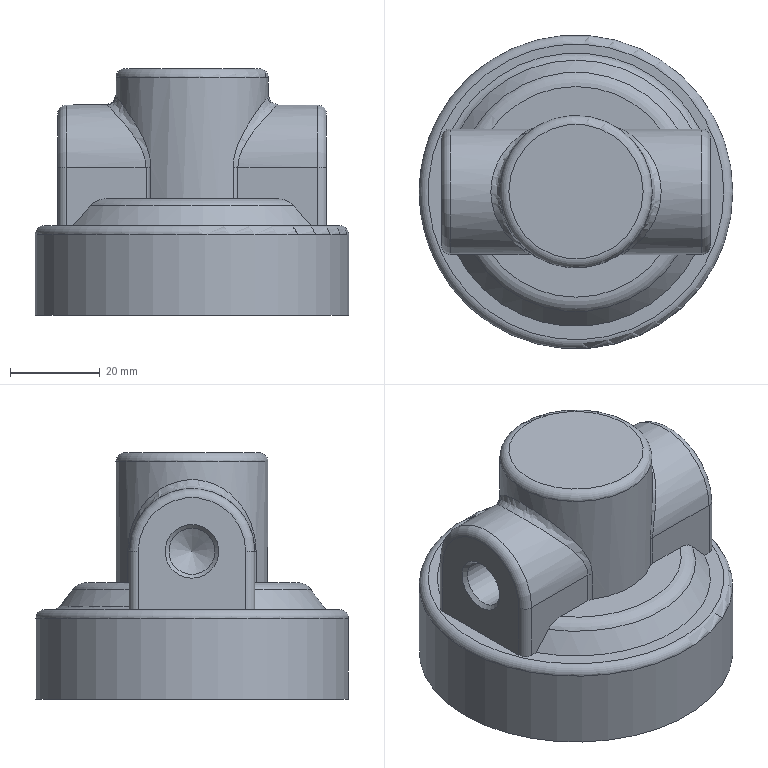Part | NX | features CYLINDER 5, HOLE PACKAGE 5, SIMPLE HOLE 5, SYMBOLIC_THREAD 4, BLEND 3, DATUM_CSYS 2, BLOCK 1, SKETCH 1, SWP104 1 | 1 solid | 51 faces | box 70 x 70 x 55 mm | volume 79994 mm3 | cylinder 19 | plane 14 | cone 9 | torus 7 | spline 2 | commonest cylinder face diameters 4 x8 10.3 x2 28 x2 3 x1 8.5 x1 34 x1
STEP:
#1=CARTESIAN_POINT('',(17.,0.,53.));
#2=VERTEX_POINT('',#1);
#3=CARTESIAN_POINT('',(0.,0.,53.));
#4=DIRECTION('',(0.,0.,1.));
#5=DIRECTION('',(1.,0.,0.));
#6=AXIS2_PLACEMENT_3D('',#3,#4,#5);
#7=CIRCLE('',#6,17.);
#8=EDGE_CURVE('',#2,#2,#7,.F.);
#9=ORIENTED_EDGE('',*,*,#8,.T.);
#10=EDGE_LOOP('',(#9));
#11=FACE_BOUND('',#10,.T.);
#12=CARTESIAN_POINT('',(9.168,-14.316,33.));
#13=VERTEX_POINT('',#12);
#14=CARTESIAN_POINT('',(9.168,14.316,33.));
#15=VERTEX_POINT('',#14);
#16=CARTESIAN_POINT('',(9.168,-14.316,33.));
#17=CARTESIAN_POINT('',(9.168,-14.316,35.135));
#18=CARTESIAN_POINT('',(10.446,-13.543,39.204));
#19=CARTESIAN_POINT('',(13.437,-10.75,44.088));
#20=CARTESIAN_POINT('',(16.145,-6.304,47.881));
#21=CARTESIAN_POINT('',(17.424,-0.02479,49.554));
#22=CARTESIAN_POINT('',(16.161,6.269,47.902));
#23=CARTESIAN_POINT('',(13.45,10.736,44.107));
#24=CARTESIAN_POINT('',(10.454,13.537,39.226));
#25=CARTESIAN_POINT('',(9.168,14.316,35.135));
#26=CARTESIAN_POINT('',(9.168,14.316,33.));
#27=B_SPLINE_CURVE_WITH_KNOTS('',3,(#16,#17,#18,#19,#20,#21,#22,#23,#24,#25,#26),.UNSPECIFIED.,.F.,.F.,(4,1,1,1,1,1,1,1,4),(0.,0.006316,0.01263,0.01895,0.02527,0.03158,0.0379,0.04422,0.05053),.UNSPECIFIED.);
#28=EDGE_CURVE('',#13,#15,#27,.T.);
#29=ORIENTED_EDGE('',*,*,#28,.T.);
#30=CARTESIAN_POINT('',(9.168,14.316,26.));
#31=VERTEX_POINT('',#30);
#32=CARTESIAN_POINT('',(9.168,14.316,0.));
#33=DIRECTION('',(0.,0.,1.));
#34=VECTOR('',#33,1000.);
#35=LINE('',#32,#34);
#36=EDGE_CURVE('',#15,#31,#35,.F.);
#37=ORIENTED_EDGE('',*,*,#36,.T.);
#38=CARTESIAN_POINT('',(-9.168,14.316,26.));
#39=VERTEX_POINT('',#38);
#40=CARTESIAN_POINT('',(0.,0.,26.));
#41=DIRECTION('',(0.,0.,-1.));
#42=DIRECTION('',(-1.,0.,0.));
#43=AXIS2_PLACEMENT_3D('',#40,#41,#42);
#44=CIRCLE('',#43,17.);
#45=EDGE_CURVE('',#31,#39,#44,.F.);
#46=ORIENTED_EDGE('',*,*,#45,.T.);
#47=CARTESIAN_POINT('',(-9.168,14.316,33.));
#48=VERTEX_POINT('',#47);
#49=CARTESIAN_POINT('',(-9.168,14.316,0.));
#50=DIRECTION('',(0.,0.,1.));
#51=VECTOR('',#50,1000.);
#52=LINE('',#49,#51);
#53=EDGE_CURVE('',#39,#48,#52,.T.);
#54=ORIENTED_EDGE('',*,*,#53,.T.);
#55=CARTESIAN_POINT('',(-9.168,-14.316,33.));
#56=VERTEX_POINT('',#55);
#57=CARTESIAN_POINT('',(-9.168,14.316,33.));
#58=CARTESIAN_POINT('',(-9.168,14.316,35.135));
#59=CARTESIAN_POINT('',(-10.446,13.543,39.204));
#60=CARTESIAN_POINT('',(-13.437,10.75,44.088));
#61=CARTESIAN_POINT('',(-16.145,6.304,47.881));
#62=CARTESIAN_POINT('',(-17.424,0.02479,49.554));
#63=CARTESIAN_POINT('',(-16.161,-6.269,47.902));
#64=CARTESIAN_POINT('',(-13.45,-10.736,44.107));
#65=CARTESIAN_POINT('',(-10.454,-13.537,39.226));
#66=CARTESIAN_POINT('',(-9.168,-14.316,35.135));
#67=CARTESIAN_POINT('',(-9.168,-14.316,33.));
#68=B_SPLINE_CURVE_WITH_KNOTS('',3,(#57,#58,#59,#60,#61,#62,#63,#64,#65,#66,#67),.UNSPECIFIED.,.F.,.F.,(4,1,1,1,1,1,1,1,4),(0.,0.006316,0.01263,0.01895,0.02527,0.03158,0.0379,0.04422,0.05053),.UNSPECIFIED.);
#69=EDGE_CURVE('',#48,#56,#68,.T.);
#70=ORIENTED_EDGE('',*,*,#69,.T.);
#71=CARTESIAN_POINT('',(-9.168,-14.316,26.));
#72=VERTEX_POINT('',#71);
#73=CARTESIAN_POINT('',(-9.168,-14.316,0.));
#74=DIRECTION('',(0.,0.,1.));
#75=VECTOR('',#74,1000.);
#76=LINE('',#73,#75);
#77=EDGE_CURVE('',#56,#72,#76,.F.);
#78=ORIENTED_EDGE('',*,*,#77,.T.);
#79=CARTESIAN_POINT('',(9.168,-14.316,26.));
#80=VERTEX_POINT('',#79);
#81=CARTESIAN_POINT('',(0.,0.,26.));
#82=DIRECTION('',(0.,0.,-1.));
#83=DIRECTION('',(-1.,0.,0.));
#84=AXIS2_PLACEMENT_3D('',#81,#82,#83);
#85=CIRCLE('',#84,17.);
#86=EDGE_CURVE('',#72,#80,#85,.F.);
#87=ORIENTED_EDGE('',*,*,#86,.T.);
#88=CARTESIAN_POINT('',(9.168,-14.316,0.));
#89=DIRECTION('',(0.,0.,1.));
#90=VECTOR('',#89,1000.);
#91=LINE('',#88,#90);
#92=EDGE_CURVE('',#80,#13,#91,.T.);
#93=ORIENTED_EDGE('',*,*,#92,.T.);
#94=EDGE_LOOP('',(#29,#37,#46,#54,#70,#78,#87,#93));
#95=FACE_BOUND('',#94,.T.);
#96=CARTESIAN_POINT('',(0.,0.,0.));
#97=DIRECTION('',(0.,0.,1.));
#98=DIRECTION('',(1.,0.,0.));
#99=AXIS2_PLACEMENT_3D('',#96,#97,#98);
#100=CYLINDRICAL_SURFACE('',#99,17.);
#101=ADVANCED_FACE('',(#11,#95),#100,.T.);
#102=CARTESIAN_POINT('',(26.533,-14.,20.));
#103=VERTEX_POINT('',#102);
#104=CARTESIAN_POINT('',(28.,-14.,20.));
#105=VERTEX_POINT('',#104);
#106=CARTESIAN_POINT('',(0.,-14.,20.));
#107=DIRECTION('',(1.,0.,0.));
#108=VECTOR('',#107,1000.);
#109=LINE('',#106,#108);
#110=EDGE_CURVE('',#103,#105,#109,.T.);
#111=ORIENTED_EDGE('',*,*,#110,.T.);
#112=CARTESIAN_POINT('',(28.,-14.,33.));
#113=VERTEX_POINT('',#112);
#114=CARTESIAN_POINT('',(28.,-14.,0.));
#115=DIRECTION('',(0.,0.,1.));
#116=VECTOR('',#115,1000.);
#117=LINE('',#114,#116);
#118=EDGE_CURVE('',#105,#113,#117,.T.);
#119=ORIENTED_EDGE('',*,*,#118,.T.);
#120=CARTESIAN_POINT('',(10.247,-14.,33.));
#121=VERTEX_POINT('',#120);
#122=CARTESIAN_POINT('',(0.,-14.,33.));
#123=DIRECTION('',(-1.,0.,0.));
#124=VECTOR('',#123,1000.);
#125=LINE('',#122,#124);
#126=EDGE_CURVE('',#113,#121,#125,.T.);
#127=ORIENTED_EDGE('',*,*,#126,.T.);
#128=CARTESIAN_POINT('',(10.247,-14.,26.));
#129=VERTEX_POINT('',#128);
#130=CARTESIAN_POINT('',(10.247,-14.,26.));
#131=DIRECTION('',(0.,0.,-1.));
#132=VECTOR('',#131,1000.);
#133=LINE('',#130,#132);
#134=EDGE_CURVE('',#121,#129,#133,.T.);
#135=ORIENTED_EDGE('',*,*,#134,.T.);
#136=CARTESIAN_POINT('',(18.875,-14.,26.));
#137=VERTEX_POINT('',#136);
#138=CARTESIAN_POINT('',(0.,-14.,26.));
#139=DIRECTION('',(1.,0.,0.));
#140=VECTOR('',#139,1000.);
#141=LINE('',#138,#140);
#142=EDGE_CURVE('',#129,#137,#141,.T.);
#143=ORIENTED_EDGE('',*,*,#142,.T.);
#144=CARTESIAN_POINT('',(22.735,-14.,24.4));
#145=VERTEX_POINT('',#144);
#146=CARTESIAN_POINT('',(18.875,-14.,26.));
#147=CARTESIAN_POINT('',(20.32,-14.,26.));
#148=CARTESIAN_POINT('',(21.777,-14.,25.488));
#149=CARTESIAN_POINT('',(22.735,-14.,24.4));
#150=B_SPLINE_CURVE_WITH_KNOTS('',3,(#146,#147,#148,#149),.UNSPECIFIED.,.F.,.F.,(4,4),(0.,0.00427),.UNSPECIFIED.);
#151=EDGE_CURVE('',#137,#145,#150,.T.);
#152=ORIENTED_EDGE('',*,*,#151,.T.);
#153=CARTESIAN_POINT('',(22.735,-14.,24.4));
#154=CARTESIAN_POINT('',(24.016,-14.,22.946));
#155=CARTESIAN_POINT('',(25.28,-14.,21.477));
#156=CARTESIAN_POINT('',(26.533,-14.,20.));
#157=B_SPLINE_CURVE_WITH_KNOTS('',3,(#153,#154,#155,#156),.UNSPECIFIED.,.F.,.F.,(4,4),(0.01619,0.022),.UNSPECIFIED.);
#158=EDGE_CURVE('',#145,#103,#157,.T.);
#159=ORIENTED_EDGE('',*,*,#158,.T.);
#160=EDGE_LOOP('',(#111,#119,#127,#135,#143,#152,#159));
#161=FACE_BOUND('',#160,.T.);
#162=CARTESIAN_POINT('',(0.,-14.,0.));
#163=DIRECTION('',(0.,-1.,0.));
#164=DIRECTION('',(0.,0.,-1.));
#165=AXIS2_PLACEMENT_3D('',#162,#163,#164);
#166=PLANE('',#165);
#167=ADVANCED_FACE('',(#161),#166,.T.);
#168=CARTESIAN_POINT('',(10.247,14.,33.));
#169=VERTEX_POINT('',#168);
#170=CARTESIAN_POINT('',(28.,14.,33.));
#171=VERTEX_POINT('',#170);
#172=CARTESIAN_POINT('',(0.,14.,33.));
#173=DIRECTION('',(1.,0.,0.));
#174=VECTOR('',#173,1000.);
#175=LINE('',#172,#174);
#176=EDGE_CURVE('',#169,#171,#175,.T.);
#177=ORIENTED_EDGE('',*,*,#176,.T.);
#178=CARTESIAN_POINT('',(28.,14.,20.));
#179=VERTEX_POINT('',#178);
#180=CARTESIAN_POINT('',(28.,14.,0.));
#181=DIRECTION('',(0.,0.,1.));
#182=VECTOR('',#181,1000.);
#183=LINE('',#180,#182);
#184=EDGE_CURVE('',#171,#179,#183,.F.);
#185=ORIENTED_EDGE('',*,*,#184,.T.);
#186=CARTESIAN_POINT('',(27.659,14.,20.));
#187=VERTEX_POINT('',#186);
#188=CARTESIAN_POINT('',(0.,14.,20.));
#189=DIRECTION('',(-1.,0.,0.));
#190=VECTOR('',#189,1000.);
#191=LINE('',#188,#190);
#192=EDGE_CURVE('',#179,#187,#191,.T.);
#193=ORIENTED_EDGE('',*,*,#192,.T.);
#194=CARTESIAN_POINT('',(25.853,14.,20.8));
#195=VERTEX_POINT('',#194);
#196=CARTESIAN_POINT('',(27.659,14.,20.));
#197=CARTESIAN_POINT('',(26.974,14.,20.));
#198=CARTESIAN_POINT('',(26.298,14.,20.278));
#199=CARTESIAN_POINT('',(25.853,14.,20.8));
#200=B_SPLINE_CURVE_WITH_KNOTS('',3,(#196,#197,#198,#199),.UNSPECIFIED.,.F.,.F.,(4,4),(0.,0.002025),.UNSPECIFIED.);
#201=EDGE_CURVE('',#187,#195,#200,.T.);
#202=ORIENTED_EDGE('',*,*,#201,.T.);
#203=CARTESIAN_POINT('',(22.735,14.,24.4));
#204=VERTEX_POINT('',#203);
#205=CARTESIAN_POINT('',(25.853,14.,20.8));
#206=CARTESIAN_POINT('',(24.823,14.,22.008));
#207=CARTESIAN_POINT('',(23.784,14.,23.209));
#208=CARTESIAN_POINT('',(22.735,14.,24.4));
#209=B_SPLINE_CURVE_WITH_KNOTS('',3,(#205,#206,#207,#208),.UNSPECIFIED.,.F.,.F.,(4,4),(0.03,0.03477),.UNSPECIFIED.);
#210=EDGE_CURVE('',#195,#204,#209,.T.);
#211=ORIENTED_EDGE('',*,*,#210,.T.);
#212=CARTESIAN_POINT('',(18.875,14.,26.));
#213=VERTEX_POINT('',#212);
#214=CARTESIAN_POINT('',(22.735,14.,24.4));
#215=CARTESIAN_POINT('',(21.778,14.,25.487));
#216=CARTESIAN_POINT('',(20.318,14.,26.));
#217=CARTESIAN_POINT('',(18.875,14.,26.));
#218=B_SPLINE_CURVE_WITH_KNOTS('',3,(#214,#215,#216,#217),.UNSPECIFIED.,.F.,.F.,(4,4),(0.,0.004276),.UNSPECIFIED.);
#219=EDGE_CURVE('',#204,#213,#218,.T.);
#220=ORIENTED_EDGE('',*,*,#219,.T.);
#221=CARTESIAN_POINT('',(10.247,14.,26.));
#222=VERTEX_POINT('',#221);
#223=CARTESIAN_POINT('',(0.,14.,26.));
#224=DIRECTION('',(-1.,0.,0.));
#225=VECTOR('',#224,1000.);
#226=LINE('',#223,#225);
#227=EDGE_CURVE('',#213,#222,#226,.T.);
#228=ORIENTED_EDGE('',*,*,#227,.T.);
#229=CARTESIAN_POINT('',(10.247,14.,33.));
#230=DIRECTION('',(0.,0.,-1.));
#231=VECTOR('',#230,1000.);
#232=LINE('',#229,#231);
#233=EDGE_CURVE('',#222,#169,#232,.F.);
#234=ORIENTED_EDGE('',*,*,#233,.T.);
#235=EDGE_LOOP('',(#177,#185,#193,#202,#211,#220,#228,#234));
#236=FACE_BOUND('',#235,.T.);
#237=CARTESIAN_POINT('',(0.,14.,0.));
#238=DIRECTION('',(0.,1.,0.));
#239=DIRECTION('',(0.,0.,1.));
#240=AXIS2_PLACEMENT_3D('',#237,#238,#239);
#241=PLANE('',#240);
#242=ADVANCED_FACE('',(#236),#241,.T.);
#243=CARTESIAN_POINT('',(-27.659,14.,20.));
#244=VERTEX_POINT('',#243);
#245=CARTESIAN_POINT('',(-28.,14.,20.));
#246=VERTEX_POINT('',#245);
#247=CARTESIAN_POINT('',(0.,14.,20.));
#248=DIRECTION('',(-1.,0.,0.));
#249=VECTOR('',#248,1000.);
#250=LINE('',#247,#249);
#251=EDGE_CURVE('',#244,#246,#250,.T.);
#252=ORIENTED_EDGE('',*,*,#251,.T.);
#253=CARTESIAN_POINT('',(-28.,14.,33.));
#254=VERTEX_POINT('',#253);
#255=CARTESIAN_POINT('',(-28.,14.,0.));
#256=DIRECTION('',(0.,0.,1.));
#257=VECTOR('',#256,1000.);
#258=LINE('',#255,#257);
#259=EDGE_CURVE('',#246,#254,#258,.T.);
#260=ORIENTED_EDGE('',*,*,#259,.T.);
#261=CARTESIAN_POINT('',(-10.247,14.,33.));
#262=VERTEX_POINT('',#261);
#263=CARTESIAN_POINT('',(0.,14.,33.));
#264=DIRECTION('',(1.,0.,0.));
#265=VECTOR('',#264,1000.);
#266=LINE('',#263,#265);
#267=EDGE_CURVE('',#254,#262,#266,.T.);
#268=ORIENTED_EDGE('',*,*,#267,.T.);
#269=CARTESIAN_POINT('',(-10.247,14.,26.));
#270=VERTEX_POINT('',#269);
#271=CARTESIAN_POINT('',(-10.247,14.,26.));
#272=DIRECTION('',(0.,0.,-1.));
#273=VECTOR('',#272,1000.);
#274=LINE('',#271,#273);
#275=EDGE_CURVE('',#262,#270,#274,.T.);
#276=ORIENTED_EDGE('',*,*,#275,.T.);
#277=CARTESIAN_POINT('',(-18.875,14.,26.));
#278=VERTEX_POINT('',#277);
#279=CARTESIAN_POINT('',(0.,14.,26.));
#280=DIRECTION('',(-1.,0.,0.));
#281=VECTOR('',#280,1000.);
#282=LINE('',#279,#281);
#283=EDGE_CURVE('',#270,#278,#282,.T.);
#284=ORIENTED_EDGE('',*,*,#283,.T.);
#285=CARTESIAN_POINT('',(-22.735,14.,24.4));
#286=VERTEX_POINT('',#285);
#287=CARTESIAN_POINT('',(-18.875,14.,26.));
#288=CARTESIAN_POINT('',(-20.32,14.,26.));
#289=CARTESIAN_POINT('',(-21.777,14.,25.488));
#290=CARTESIAN_POINT('',(-22.735,14.,24.4));
#291=B_SPLINE_CURVE_WITH_KNOTS('',3,(#287,#288,#289,#290),.UNSPECIFIED.,.F.,.F.,(4,4),(0.,0.00427),.UNSPECIFIED.);
#292=EDGE_CURVE('',#278,#286,#291,.T.);
#293=ORIENTED_EDGE('',*,*,#292,.T.);
#294=CARTESIAN_POINT('',(-25.853,14.,20.8));
#295=VERTEX_POINT('',#294);
#296=CARTESIAN_POINT('',(-22.735,14.,24.4));
#297=CARTESIAN_POINT('',(-23.784,14.,23.209));
#298=CARTESIAN_POINT('',(-24.822,14.,22.008));
#299=CARTESIAN_POINT('',(-25.853,14.,20.8));
#300=B_SPLINE_CURVE_WITH_KNOTS('',3,(#296,#297,#298,#299),.UNSPECIFIED.,.F.,.F.,(4,4),(0.01405,0.01881),.UNSPECIFIED.);
#301=EDGE_CURVE('',#286,#295,#300,.T.);
#302=ORIENTED_EDGE('',*,*,#301,.T.);
#303=CARTESIAN_POINT('',(-25.853,14.,20.8));
#304=CARTESIAN_POINT('',(-26.297,14.,20.279));
#305=CARTESIAN_POINT('',(-26.975,14.,20.));
#306=CARTESIAN_POINT('',(-27.659,14.,20.));
#307=B_SPLINE_CURVE_WITH_KNOTS('',3,(#303,#304,#305,#306),.UNSPECIFIED.,.F.,.F.,(4,4),(0.,0.002024),.UNSPECIFIED.);
#308=EDGE_CURVE('',#295,#244,#307,.T.);
#309=ORIENTED_EDGE('',*,*,#308,.T.);
#310=EDGE_LOOP('',(#252,#260,#268,#276,#284,#293,#302,#309));
#311=FACE_BOUND('',#310,.T.);
#312=CARTESIAN_POINT('',(0.,14.,0.));
#313=DIRECTION('',(0.,1.,0.));
#314=DIRECTION('',(0.,0.,1.));
#315=AXIS2_PLACEMENT_3D('',#312,#313,#314);
#316=PLANE('',#315);
#317=ADVANCED_FACE('',(#311),#316,.T.);
#318=CARTESIAN_POINT('',(-10.247,-14.,33.));
#319=VERTEX_POINT('',#318);
#320=CARTESIAN_POINT('',(-28.,-14.,33.));
#321=VERTEX_POINT('',#320);
#322=CARTESIAN_POINT('',(0.,-14.,33.));
#323=DIRECTION('',(-1.,0.,0.));
#324=VECTOR('',#323,1000.);
#325=LINE('',#322,#324);
#326=EDGE_CURVE('',#319,#321,#325,.T.);
#327=ORIENTED_EDGE('',*,*,#326,.T.);
#328=CARTESIAN_POINT('',(-28.,-14.,20.));
#329=VERTEX_POINT('',#328);
#330=CARTESIAN_POINT('',(-28.,-14.,0.));
#331=DIRECTION('',(0.,0.,1.));
#332=VECTOR('',#331,1000.);
#333=LINE('',#330,#332);
#334=EDGE_CURVE('',#321,#329,#333,.F.);
#335=ORIENTED_EDGE('',*,*,#334,.T.);
#336=CARTESIAN_POINT('',(-26.533,-14.,20.));
#337=VERTEX_POINT('',#336);
#338=CARTESIAN_POINT('',(0.,-14.,20.));
#339=DIRECTION('',(1.,0.,0.));
#340=VECTOR('',#339,1000.);
#341=LINE('',#338,#340);
#342=EDGE_CURVE('',#329,#337,#341,.T.);
#343=ORIENTED_EDGE('',*,*,#342,.T.);
#344=CARTESIAN_POINT('',(-22.735,-14.,24.4));
#345=VERTEX_POINT('',#344);
#346=CARTESIAN_POINT('',(-26.533,-14.,20.));
#347=CARTESIAN_POINT('',(-25.28,-14.,21.478));
#348=CARTESIAN_POINT('',(-24.015,-14.,22.947));
#349=CARTESIAN_POINT('',(-22.735,-14.,24.4));
#350=B_SPLINE_CURVE_WITH_KNOTS('',3,(#346,#347,#348,#349),.UNSPECIFIED.,.F.,.F.,(4,4),(0.0346,0.04041),.UNSPECIFIED.);
#351=EDGE_CURVE('',#337,#345,#350,.T.);
#352=ORIENTED_EDGE('',*,*,#351,.T.);
#353=CARTESIAN_POINT('',(-18.875,-14.,26.));
#354=VERTEX_POINT('',#353);
#355=CARTESIAN_POINT('',(-22.735,-14.,24.4));
#356=CARTESIAN_POINT('',(-21.778,-14.,25.487));
#357=CARTESIAN_POINT('',(-20.318,-14.,26.));
#358=CARTESIAN_POINT('',(-18.875,-14.,26.));
#359=B_SPLINE_CURVE_WITH_KNOTS('',3,(#355,#356,#357,#358),.UNSPECIFIED.,.F.,.F.,(4,4),(0.,0.004276),.UNSPECIFIED.);
#360=EDGE_CURVE('',#345,#354,#359,.T.);
#361=ORIENTED_EDGE('',*,*,#360,.T.);
#362=CARTESIAN_POINT('',(-10.247,-14.,26.));
#363=VERTEX_POINT('',#362);
#364=CARTESIAN_POINT('',(0.,-14.,26.));
#365=DIRECTION('',(1.,0.,0.));
#366=VECTOR('',#365,1000.);
#367=LINE('',#364,#366);
#368=EDGE_CURVE('',#354,#363,#367,.T.);
#369=ORIENTED_EDGE('',*,*,#368,.T.);
#370=CARTESIAN_POINT('',(-10.247,-14.,33.));
#371=DIRECTION('',(0.,0.,-1.));
#372=VECTOR('',#371,1000.);
#373=LINE('',#370,#372);
#374=EDGE_CURVE('',#363,#319,#373,.F.);
#375=ORIENTED_EDGE('',*,*,#374,.T.);
#376=EDGE_LOOP('',(#327,#335,#343,#352,#361,#369,#375));
#377=FACE_BOUND('',#376,.T.);
#378=CARTESIAN_POINT('',(0.,-14.,0.));
#379=DIRECTION('',(0.,-1.,0.));
#380=DIRECTION('',(0.,0.,-1.));
#381=AXIS2_PLACEMENT_3D('',#378,#379,#380);
#382=PLANE('',#381);
#383=ADVANCED_FACE('',(#377),#382,.T.);
#384=CARTESIAN_POINT('',(33.,0.,20.));
#385=VERTEX_POINT('',#384);
#386=CARTESIAN_POINT('',(0.,0.,20.));
#387=DIRECTION('',(0.,0.,1.));
#388=DIRECTION('',(1.,0.,0.));
#389=AXIS2_PLACEMENT_3D('',#386,#387,#388);
#390=CIRCLE('',#389,33.);
#391=EDGE_CURVE('',#385,#385,#390,.T.);
#392=ORIENTED_EDGE('',*,*,#391,.T.);
#393=EDGE_LOOP('',(#392));
#394=FACE_BOUND('',#393,.T.);
#395=CARTESIAN_POINT('',(-30.,12.,20.));
#396=VERTEX_POINT('',#395);
#397=CARTESIAN_POINT('',(-30.,0.,20.));
#398=VERTEX_POINT('',#397);
#399=CARTESIAN_POINT('',(-30.,0.,20.));
#400=DIRECTION('',(0.,-1.,0.));
#401=VECTOR('',#400,1000.);
#402=LINE('',#399,#401);
#403=EDGE_CURVE('',#396,#398,#402,.T.);
#404=ORIENTED_EDGE('',*,*,#403,.F.);
#405=CARTESIAN_POINT('',(-28.,12.,20.));
#406=DIRECTION('',(0.,0.,1.));
#407=DIRECTION('',(1.,0.,0.));
#408=AXIS2_PLACEMENT_3D('',#405,#406,#407);
#409=CIRCLE('',#408,2.);
#410=EDGE_CURVE('',#396,#246,#409,.F.);
#411=ORIENTED_EDGE('',*,*,#410,.T.);
#412=ORIENTED_EDGE('',*,*,#251,.F.);
#413=CARTESIAN_POINT('',(0.,0.,20.));
#414=DIRECTION('',(0.,0.,1.));
#415=DIRECTION('',(1.,0.,0.));
#416=AXIS2_PLACEMENT_3D('',#413,#414,#415);
#417=CIRCLE('',#416,31.);
#418=EDGE_CURVE('',#244,#187,#417,.F.);
#419=ORIENTED_EDGE('',*,*,#418,.T.);
#420=ORIENTED_EDGE('',*,*,#192,.F.);
#421=CARTESIAN_POINT('',(30.,12.,20.));
#422=VERTEX_POINT('',#421);
#423=CARTESIAN_POINT('',(28.,12.,20.));
#424=DIRECTION('',(0.,0.,1.));
#425=DIRECTION('',(1.,0.,0.));
#426=AXIS2_PLACEMENT_3D('',#423,#424,#425);
#427=CIRCLE('',#426,2.);
#428=EDGE_CURVE('',#179,#422,#427,.F.);
#429=ORIENTED_EDGE('',*,*,#428,.T.);
#430=CARTESIAN_POINT('',(30.,0.,20.));
#431=VERTEX_POINT('',#430);
#432=CARTESIAN_POINT('',(30.,0.,20.));
#433=DIRECTION('',(0.,1.,0.));
#434=VECTOR('',#433,1000.);
#435=LINE('',#432,#434);
#436=EDGE_CURVE('',#431,#422,#435,.T.);
#437=ORIENTED_EDGE('',*,*,#436,.F.);
#438=CARTESIAN_POINT('',(30.,-12.,20.));
#439=VERTEX_POINT('',#438);
#440=CARTESIAN_POINT('',(30.,0.,20.));
#441=DIRECTION('',(0.,1.,0.));
#442=VECTOR('',#441,1000.);
#443=LINE('',#440,#442);
#444=EDGE_CURVE('',#439,#431,#443,.T.);
#445=ORIENTED_EDGE('',*,*,#444,.F.);
#446=CARTESIAN_POINT('',(28.,-12.,20.));
#447=DIRECTION('',(0.,0.,1.));
#448=DIRECTION('',(1.,0.,0.));
#449=AXIS2_PLACEMENT_3D('',#446,#447,#448);
#450=CIRCLE('',#449,2.);
#451=EDGE_CURVE('',#439,#105,#450,.F.);
#452=ORIENTED_EDGE('',*,*,#451,.T.);
#453=ORIENTED_EDGE('',*,*,#110,.F.);
#454=CARTESIAN_POINT('',(0.,0.,20.));
#455=DIRECTION('',(0.,0.,1.));
#456=DIRECTION('',(1.,0.,0.));
#457=AXIS2_PLACEMENT_3D('',#454,#455,#456);
#458=CIRCLE('',#457,30.);
#459=EDGE_CURVE('',#337,#103,#458,.T.);
#460=ORIENTED_EDGE('',*,*,#459,.F.);
#461=ORIENTED_EDGE('',*,*,#342,.F.);
#462=CARTESIAN_POINT('',(-30.,-12.,20.));
#463=VERTEX_POINT('',#462);
#464=CARTESIAN_POINT('',(-28.,-12.,20.));
#465=DIRECTION('',(0.,0.,1.));
#466=DIRECTION('',(1.,0.,0.));
#467=AXIS2_PLACEMENT_3D('',#464,#465,#466);
#468=CIRCLE('',#467,2.);
#469=EDGE_CURVE('',#329,#463,#468,.F.);
#470=ORIENTED_EDGE('',*,*,#469,.T.);
#471=CARTESIAN_POINT('',(-30.,0.,20.));
#472=DIRECTION('',(0.,-1.,0.));
#473=VECTOR('',#472,1000.);
#474=LINE('',#471,#473);
#475=EDGE_CURVE('',#398,#463,#474,.T.);
#476=ORIENTED_EDGE('',*,*,#475,.F.);
#477=EDGE_LOOP('',(#404,#411,#412,#419,#420,#429,#437,#445,#452,#453,#460,#461,#470,#476));
#478=FACE_BOUND('',#477,.T.);
#479=CARTESIAN_POINT('',(0.,0.,20.));
#480=DIRECTION('',(0.,0.,1.));
#481=DIRECTION('',(1.,0.,0.));
#482=AXIS2_PLACEMENT_3D('',#479,#480,#481);
#483=PLANE('',#482);
#484=ADVANCED_FACE('',(#394,#478),#483,.T.);
#485=CARTESIAN_POINT('',(-30.,0.,0.));
#486=VERTEX_POINT('',#485);
#487=CARTESIAN_POINT('',(0.,0.,0.));
#488=DIRECTION('',(0.,0.,-1.));
#489=DIRECTION('',(-1.,0.,0.));
#490=AXIS2_PLACEMENT_3D('',#487,#488,#489);
#491=CIRCLE('',#490,30.);
#492=EDGE_CURVE('',#486,#486,#491,.F.);
#493=ORIENTED_EDGE('',*,*,#492,.T.);
#494=EDGE_LOOP('',(#493));
#495=FACE_BOUND('',#494,.T.);
#496=CARTESIAN_POINT('',(35.,0.,0.));
#497=VERTEX_POINT('',#496);
#498=CARTESIAN_POINT('',(0.,0.,0.));
#499=DIRECTION('',(0.,0.,1.));
#500=DIRECTION('',(1.,0.,0.));
#501=AXIS2_PLACEMENT_3D('',#498,#499,#500);
#502=CIRCLE('',#501,35.);
#503=EDGE_CURVE('',#497,#497,#502,.T.);
#504=ORIENTED_EDGE('',*,*,#503,.F.);
#505=EDGE_LOOP('',(#504));
#506=FACE_BOUND('',#505,.T.);
#507=CARTESIAN_POINT('',(0.,0.,0.));
#508=DIRECTION('',(0.,0.,-1.));
#509=DIRECTION('',(-1.,0.,0.));
#510=AXIS2_PLACEMENT_3D('',#507,#508,#509);
#511=PLANE('',#510);
#512=ADVANCED_FACE('',(#495,#506),#511,.T.);
#513=CARTESIAN_POINT('',(35.,0.,18.));
#514=VERTEX_POINT('',#513);
#515=CARTESIAN_POINT('',(0.,0.,18.));
#516=DIRECTION('',(0.,0.,1.));
#517=DIRECTION('',(1.,0.,0.));
#518=AXIS2_PLACEMENT_3D('',#515,#516,#517);
#519=CIRCLE('',#518,35.);
#520=EDGE_CURVE('',#514,#514,#519,.F.);
#521=ORIENTED_EDGE('',*,*,#520,.T.);
#522=EDGE_LOOP('',(#521));
#523=FACE_BOUND('',#522,.T.);
#524=ORIENTED_EDGE('',*,*,#503,.T.);
#525=EDGE_LOOP('',(#524));
#526=FACE_BOUND('',#525,.T.);
#527=CARTESIAN_POINT('',(0.,0.,0.));
#528=DIRECTION('',(0.,0.,1.));
#529=DIRECTION('',(1.,0.,0.));
#530=AXIS2_PLACEMENT_3D('',#527,#528,#529);
#531=CYLINDRICAL_SURFACE('',#530,35.);
#532=ADVANCED_FACE('',(#523,#526),#531,.T.);
#533=CARTESIAN_POINT('',(15.,0.,55.));
#534=VERTEX_POINT('',#533);
#535=CARTESIAN_POINT('',(0.,0.,55.));
#536=DIRECTION('',(0.,0.,1.));
#537=DIRECTION('',(1.,0.,0.));
#538=AXIS2_PLACEMENT_3D('',#535,#536,#537);
#539=CIRCLE('',#538,15.);
#540=EDGE_CURVE('',#534,#534,#539,.T.);
#541=ORIENTED_EDGE('',*,*,#540,.T.);
#542=EDGE_LOOP('',(#541));
#543=FACE_BOUND('',#542,.T.);
#544=CARTESIAN_POINT('',(0.,0.,55.));
#545=DIRECTION('',(0.,0.,1.));
#546=DIRECTION('',(1.,0.,0.));
#547=AXIS2_PLACEMENT_3D('',#544,#545,#546);
#548=PLANE('',#547);
#549=ADVANCED_FACE('',(#543),#548,.T.);
#550=CARTESIAN_POINT('',(30.,0.,27.));
#551=VERTEX_POINT('',#550);
#552=CARTESIAN_POINT('',(30.,0.,33.));
#553=DIRECTION('',(1.,0.,0.));
#554=DIRECTION('',(0.,0.,-1.));
#555=AXIS2_PLACEMENT_3D('',#552,#553,#554);
#556=CIRCLE('',#555,6.);
#557=EDGE_CURVE('',#551,#551,#556,.F.);
#558=ORIENTED_EDGE('',*,*,#557,.T.);
#559=EDGE_LOOP('',(#558));
#560=FACE_BOUND('',#559,.T.);
#561=CARTESIAN_POINT('',(30.,12.,33.));
#562=VERTEX_POINT('',#561);
#563=CARTESIAN_POINT('',(30.,-12.,33.));
#564=VERTEX_POINT('',#563);
#565=CARTESIAN_POINT('',(30.,0.,33.));
#566=DIRECTION('',(1.,0.,0.));
#567=DIRECTION('',(0.,0.,-1.));
#568=AXIS2_PLACEMENT_3D('',#565,#566,#567);
#569=CIRCLE('',#568,12.);
#570=EDGE_CURVE('',#562,#564,#569,.T.);
#571=ORIENTED_EDGE('',*,*,#570,.T.);
#572=CARTESIAN_POINT('',(30.,-12.,0.));
#573=DIRECTION('',(0.,0.,1.));
#574=VECTOR('',#573,1000.);
#575=LINE('',#572,#574);
#576=EDGE_CURVE('',#564,#439,#575,.F.);
#577=ORIENTED_EDGE('',*,*,#576,.T.);
#578=ORIENTED_EDGE('',*,*,#444,.T.);
#579=ORIENTED_EDGE('',*,*,#436,.T.);
#580=CARTESIAN_POINT('',(30.,12.,0.));
#581=DIRECTION('',(0.,0.,1.));
#582=VECTOR('',#581,1000.);
#583=LINE('',#580,#582);
#584=EDGE_CURVE('',#422,#562,#583,.T.);
#585=ORIENTED_EDGE('',*,*,#584,.T.);
#586=EDGE_LOOP('',(#571,#577,#578,#579,#585));
#587=FACE_BOUND('',#586,.T.);
#588=CARTESIAN_POINT('',(30.,0.,0.));
#589=DIRECTION('',(1.,0.,0.));
#590=DIRECTION('',(0.,0.,-1.));
#591=AXIS2_PLACEMENT_3D('',#588,#589,#590);
#592=PLANE('',#591);
#593=ADVANCED_FACE('',(#560,#587),#592,.T.);
#594=CARTESIAN_POINT('',(-30.,0.,39.));
#595=VERTEX_POINT('',#594);
#596=CARTESIAN_POINT('',(-30.,0.,33.));
#597=DIRECTION('',(-1.,0.,0.));
#598=DIRECTION('',(0.,0.,1.));
#599=AXIS2_PLACEMENT_3D('',#596,#597,#598);
#600=CIRCLE('',#599,6.);
#601=EDGE_CURVE('',#595,#595,#600,.F.);
#602=ORIENTED_EDGE('',*,*,#601,.T.);
#603=EDGE_LOOP('',(#602));
#604=FACE_BOUND('',#603,.T.);
#605=CARTESIAN_POINT('',(-30.,-12.,33.));
#606=VERTEX_POINT('',#605);
#607=CARTESIAN_POINT('',(-30.,12.,33.));
#608=VERTEX_POINT('',#607);
#609=CARTESIAN_POINT('',(-30.,0.,33.));
#610=DIRECTION('',(-1.,0.,0.));
#611=DIRECTION('',(0.,0.,1.));
#612=AXIS2_PLACEMENT_3D('',#609,#610,#611);
#613=CIRCLE('',#612,12.);
#614=EDGE_CURVE('',#606,#608,#613,.T.);
#615=ORIENTED_EDGE('',*,*,#614,.T.);
#616=CARTESIAN_POINT('',(-30.,12.,0.));
#617=DIRECTION('',(0.,0.,1.));
#618=VECTOR('',#617,1000.);
#619=LINE('',#616,#618);
#620=EDGE_CURVE('',#608,#396,#619,.F.);
#621=ORIENTED_EDGE('',*,*,#620,.T.);
#622=ORIENTED_EDGE('',*,*,#403,.T.);
#623=ORIENTED_EDGE('',*,*,#475,.T.);
#624=CARTESIAN_POINT('',(-30.,-12.,0.));
#625=DIRECTION('',(0.,0.,1.));
#626=VECTOR('',#625,1000.);
#627=LINE('',#624,#626);
#628=EDGE_CURVE('',#463,#606,#627,.T.);
#629=ORIENTED_EDGE('',*,*,#628,.T.);
#630=EDGE_LOOP('',(#615,#621,#622,#623,#629));
#631=FACE_BOUND('',#630,.T.);
#632=CARTESIAN_POINT('',(-30.,0.,0.));
#633=DIRECTION('',(-1.,0.,0.));
#634=DIRECTION('',(0.,0.,1.));
#635=AXIS2_PLACEMENT_3D('',#632,#633,#634);
#636=PLANE('',#635);
#637=ADVANCED_FACE('',(#604,#631),#636,.T.);
#638=ORIENTED_EDGE('',*,*,#267,.F.);
#639=CARTESIAN_POINT('',(-28.,0.,33.));
#640=DIRECTION('',(-1.,0.,0.));
#641=DIRECTION('',(0.,0.,1.));
#642=AXIS2_PLACEMENT_3D('',#639,#640,#641);
#643=CIRCLE('',#642,14.);
#644=EDGE_CURVE('',#254,#321,#643,.F.);
#645=ORIENTED_EDGE('',*,*,#644,.T.);
#646=ORIENTED_EDGE('',*,*,#326,.F.);
#647=CARTESIAN_POINT('',(-10.247,-14.,33.));
#648=CARTESIAN_POINT('',(-10.247,-14.,35.031));
#649=CARTESIAN_POINT('',(-11.896,-13.111,38.768));
#650=CARTESIAN_POINT('',(-15.216,-10.291,42.923));
#651=CARTESIAN_POINT('',(-18.125,-5.942,46.105));
#652=CARTESIAN_POINT('',(-19.442,0.02427,47.452));
#653=CARTESIAN_POINT('',(-18.108,5.978,46.086));
#654=CARTESIAN_POINT('',(-15.201,10.306,42.907));
#655=CARTESIAN_POINT('',(-11.884,13.118,38.745));
#656=CARTESIAN_POINT('',(-10.247,14.,35.032));
#657=CARTESIAN_POINT('',(-10.247,14.,33.));
#658=B_SPLINE_CURVE_WITH_KNOTS('',3,(#647,#648,#649,#650,#651,#652,#653,#654,#655,#656,#657),.UNSPECIFIED.,.F.,.F.,(4,1,1,1,1,1,1,1,4),(0.,0.006084,0.01217,0.01825,0.02434,0.03042,0.03651,0.04259,0.04868),.UNSPECIFIED.);
#659=EDGE_CURVE('',#319,#262,#658,.T.);
#660=ORIENTED_EDGE('',*,*,#659,.T.);
#661=EDGE_LOOP('',(#638,#645,#646,#660));
#662=FACE_BOUND('',#661,.T.);
#663=CARTESIAN_POINT('',(-30.,0.,33.));
#664=DIRECTION('',(1.,0.,0.));
#665=DIRECTION('',(0.,0.,-1.));
#666=AXIS2_PLACEMENT_3D('',#663,#664,#665);
#667=CYLINDRICAL_SURFACE('',#666,14.);
#668=ADVANCED_FACE('',(#662),#667,.T.);
#669=ORIENTED_EDGE('',*,*,#126,.F.);
#670=CARTESIAN_POINT('',(28.,0.,33.));
#671=DIRECTION('',(1.,0.,0.));
#672=DIRECTION('',(0.,0.,-1.));
#673=AXIS2_PLACEMENT_3D('',#670,#671,#672);
#674=CIRCLE('',#673,14.);
#675=EDGE_CURVE('',#113,#171,#674,.F.);
#676=ORIENTED_EDGE('',*,*,#675,.T.);
#677=ORIENTED_EDGE('',*,*,#176,.F.);
#678=CARTESIAN_POINT('',(10.247,14.,33.));
#679=CARTESIAN_POINT('',(10.247,14.,35.031));
#680=CARTESIAN_POINT('',(11.896,13.111,38.768));
#681=CARTESIAN_POINT('',(15.216,10.291,42.923));
#682=CARTESIAN_POINT('',(18.125,5.942,46.105));
#683=CARTESIAN_POINT('',(19.442,-0.02427,47.452));
#684=CARTESIAN_POINT('',(18.108,-5.978,46.086));
#685=CARTESIAN_POINT('',(15.201,-10.306,42.907));
#686=CARTESIAN_POINT('',(11.884,-13.118,38.745));
#687=CARTESIAN_POINT('',(10.247,-14.,35.032));
#688=CARTESIAN_POINT('',(10.247,-14.,33.));
#689=B_SPLINE_CURVE_WITH_KNOTS('',3,(#678,#679,#680,#681,#682,#683,#684,#685,#686,#687,#688),.UNSPECIFIED.,.F.,.F.,(4,1,1,1,1,1,1,1,4),(0.,0.006084,0.01217,0.01825,0.02434,0.03042,0.03651,0.04259,0.04868),.UNSPECIFIED.);
#690=EDGE_CURVE('',#169,#121,#689,.T.);
#691=ORIENTED_EDGE('',*,*,#690,.T.);
#692=EDGE_LOOP('',(#669,#676,#677,#691));
#693=FACE_BOUND('',#692,.T.);
#694=CARTESIAN_POINT('',(-30.,0.,33.));
#695=DIRECTION('',(1.,0.,0.));
#696=DIRECTION('',(0.,0.,-1.));
#697=AXIS2_PLACEMENT_3D('',#694,#695,#696);
#698=CYLINDRICAL_SURFACE('',#697,14.);
#699=ADVANCED_FACE('',(#693),#698,.T.);
#700=ORIENTED_EDGE('',*,*,#158,.F.);
#701=CARTESIAN_POINT('',(0.,0.,24.4));
#702=DIRECTION('',(0.,0.,1.));
#703=DIRECTION('',(1.,0.,0.));
#704=AXIS2_PLACEMENT_3D('',#701,#702,#703);
#705=CIRCLE('',#704,26.7);
#706=EDGE_CURVE('',#145,#345,#705,.F.);
#707=ORIENTED_EDGE('',*,*,#706,.T.);
#708=ORIENTED_EDGE('',*,*,#351,.F.);
#709=ORIENTED_EDGE('',*,*,#459,.T.);
#710=EDGE_LOOP('',(#700,#707,#708,#709));
#711=FACE_BOUND('',#710,.T.);
#712=CARTESIAN_POINT('',(0.,0.,20.));
#713=DIRECTION('',(0.,0.,-1.));
#714=DIRECTION('',(-1.,0.,0.));
#715=AXIS2_PLACEMENT_3D('',#712,#713,#714);
#716=CONICAL_SURFACE('',#715,30.,0.6435);
#717=ADVANCED_FACE('',(#711),#716,.T.);
#718=ORIENTED_EDGE('',*,*,#142,.F.);
#719=CARTESIAN_POINT('',(10.247,-16.,26.));
#720=DIRECTION('',(0.,0.,-1.));
#721=DIRECTION('',(-1.,0.,0.));
#722=AXIS2_PLACEMENT_3D('',#719,#720,#721);
#723=CIRCLE('',#722,2.);
#724=EDGE_CURVE('',#129,#80,#723,.F.);
#725=ORIENTED_EDGE('',*,*,#724,.T.);
#726=ORIENTED_EDGE('',*,*,#86,.F.);
#727=CARTESIAN_POINT('',(-10.247,-16.,26.));
#728=DIRECTION('',(0.,0.,-1.));
#729=DIRECTION('',(-1.,0.,0.));
#730=AXIS2_PLACEMENT_3D('',#727,#728,#729);
#731=CIRCLE('',#730,2.);
#732=EDGE_CURVE('',#72,#363,#731,.F.);
#733=ORIENTED_EDGE('',*,*,#732,.T.);
#734=ORIENTED_EDGE('',*,*,#368,.F.);
#735=CARTESIAN_POINT('',(0.,0.,26.));
#736=DIRECTION('',(0.,0.,-1.));
#737=DIRECTION('',(-1.,0.,0.));
#738=AXIS2_PLACEMENT_3D('',#735,#736,#737);
#739=CIRCLE('',#738,23.5);
#740=EDGE_CURVE('',#354,#137,#739,.F.);
#741=ORIENTED_EDGE('',*,*,#740,.T.);
#742=EDGE_LOOP('',(#718,#725,#726,#733,#734,#741));
#743=FACE_BOUND('',#742,.T.);
#744=CARTESIAN_POINT('',(25.5,0.,26.));
#745=DIRECTION('',(0.,0.,-1.));
#746=DIRECTION('',(-1.,0.,0.));
#747=AXIS2_PLACEMENT_3D('',#744,#745,#746);
#748=PLANE('',#747);
#749=ADVANCED_FACE('',(#743),#748,.F.);
#750=ORIENTED_EDGE('',*,*,#45,.F.);
#751=CARTESIAN_POINT('',(10.247,16.,26.));
#752=DIRECTION('',(0.,0.,-1.));
#753=DIRECTION('',(-1.,0.,0.));
#754=AXIS2_PLACEMENT_3D('',#751,#752,#753);
#755=CIRCLE('',#754,2.);
#756=EDGE_CURVE('',#31,#222,#755,.F.);
#757=ORIENTED_EDGE('',*,*,#756,.T.);
#758=ORIENTED_EDGE('',*,*,#227,.F.);
#759=CARTESIAN_POINT('',(0.,0.,26.));
#760=DIRECTION('',(0.,0.,-1.));
#761=DIRECTION('',(-1.,0.,0.));
#762=AXIS2_PLACEMENT_3D('',#759,#760,#761);
#763=CIRCLE('',#762,23.5);
#764=EDGE_CURVE('',#213,#278,#763,.F.);
#765=ORIENTED_EDGE('',*,*,#764,.T.);
#766=ORIENTED_EDGE('',*,*,#283,.F.);
#767=CARTESIAN_POINT('',(-10.247,16.,26.));
#768=DIRECTION('',(0.,0.,-1.));
#769=DIRECTION('',(-1.,0.,0.));
#770=AXIS2_PLACEMENT_3D('',#767,#768,#769);
#771=CIRCLE('',#770,2.);
#772=EDGE_CURVE('',#270,#39,#771,.F.);
#773=ORIENTED_EDGE('',*,*,#772,.T.);
#774=EDGE_LOOP('',(#750,#757,#758,#765,#766,#773));
#775=FACE_BOUND('',#774,.T.);
#776=CARTESIAN_POINT('',(25.5,0.,26.));
#777=DIRECTION('',(0.,0.,-1.));
#778=DIRECTION('',(-1.,0.,0.));
#779=AXIS2_PLACEMENT_3D('',#776,#777,#778);
#780=PLANE('',#779);
#781=ADVANCED_FACE('',(#775),#780,.F.);
#782=ORIENTED_EDGE('',*,*,#210,.F.);
#783=CARTESIAN_POINT('',(0.,0.,20.8));
#784=DIRECTION('',(0.,0.,1.));
#785=DIRECTION('',(1.,0.,0.));
#786=AXIS2_PLACEMENT_3D('',#783,#784,#785);
#787=CIRCLE('',#786,29.4);
#788=EDGE_CURVE('',#195,#295,#787,.T.);
#789=ORIENTED_EDGE('',*,*,#788,.T.);
#790=ORIENTED_EDGE('',*,*,#301,.F.);
#791=CARTESIAN_POINT('',(0.,0.,24.4));
#792=DIRECTION('',(0.,0.,1.));
#793=DIRECTION('',(1.,0.,0.));
#794=AXIS2_PLACEMENT_3D('',#791,#792,#793);
#795=CIRCLE('',#794,26.7);
#796=EDGE_CURVE('',#286,#204,#795,.F.);
#797=ORIENTED_EDGE('',*,*,#796,.T.);
#798=EDGE_LOOP('',(#782,#789,#790,#797));
#799=FACE_BOUND('',#798,.T.);
#800=CARTESIAN_POINT('',(0.,0.,20.));
#801=DIRECTION('',(0.,0.,-1.));
#802=DIRECTION('',(-1.,0.,0.));
#803=AXIS2_PLACEMENT_3D('',#800,#801,#802);
#804=CONICAL_SURFACE('',#803,30.,0.6435);
#805=ADVANCED_FACE('',(#799),#804,.T.);
#806=ORIENTED_EDGE('',*,*,#360,.F.);
#807=ORIENTED_EDGE('',*,*,#706,.F.);
#808=ORIENTED_EDGE('',*,*,#151,.F.);
#809=ORIENTED_EDGE('',*,*,#740,.F.);
#810=EDGE_LOOP('',(#806,#807,#808,#809));
#811=FACE_BOUND('',#810,.T.);
#812=CARTESIAN_POINT('',(0.,0.,22.));
#813=DIRECTION('',(0.,0.,-1.));
#814=DIRECTION('',(-1.,0.,0.));
#815=AXIS2_PLACEMENT_3D('',#812,#813,#814);
#816=TOROIDAL_SURFACE('',#815,23.5,4.);
#817=ADVANCED_FACE('',(#811),#816,.T.);
#818=ORIENTED_EDGE('',*,*,#219,.F.);
#819=ORIENTED_EDGE('',*,*,#796,.F.);
#820=ORIENTED_EDGE('',*,*,#292,.F.);
#821=ORIENTED_EDGE('',*,*,#764,.F.);
#822=EDGE_LOOP('',(#818,#819,#820,#821));
#823=FACE_BOUND('',#822,.T.);
#824=CARTESIAN_POINT('',(0.,0.,22.));
#825=DIRECTION('',(0.,0.,-1.));
#826=DIRECTION('',(-1.,0.,0.));
#827=AXIS2_PLACEMENT_3D('',#824,#825,#826);
#828=TOROIDAL_SURFACE('',#827,23.5,4.);
#829=ADVANCED_FACE('',(#823),#828,.T.);
#830=ORIENTED_EDGE('',*,*,#428,.F.);
#831=ORIENTED_EDGE('',*,*,#184,.F.);
#832=CARTESIAN_POINT('',(28.,12.,33.));
#833=DIRECTION('',(0.,0.,1.));
#834=DIRECTION('',(1.,0.,0.));
#835=AXIS2_PLACEMENT_3D('',#832,#833,#834);
#836=CIRCLE('',#835,2.);
#837=EDGE_CURVE('',#562,#171,#836,.T.);
#838=ORIENTED_EDGE('',*,*,#837,.F.);
#839=ORIENTED_EDGE('',*,*,#584,.F.);
#840=EDGE_LOOP('',(#830,#831,#838,#839));
#841=FACE_BOUND('',#840,.T.);
#842=CARTESIAN_POINT('',(28.,12.,0.));
#843=DIRECTION('',(0.,0.,1.));
#844=DIRECTION('',(1.,0.,0.));
#845=AXIS2_PLACEMENT_3D('',#842,#843,#844);
#846=CYLINDRICAL_SURFACE('',#845,2.);
#847=ADVANCED_FACE('',(#841),#846,.T.);
#848=ORIENTED_EDGE('',*,*,#837,.T.);
#849=ORIENTED_EDGE('',*,*,#675,.F.);
#850=CARTESIAN_POINT('',(28.,-12.,33.));
#851=DIRECTION('',(0.,0.,-1.));
#852=DIRECTION('',(-1.,0.,0.));
#853=AXIS2_PLACEMENT_3D('',#850,#851,#852);
#854=CIRCLE('',#853,2.);
#855=EDGE_CURVE('',#564,#113,#854,.T.);
#856=ORIENTED_EDGE('',*,*,#855,.F.);
#857=ORIENTED_EDGE('',*,*,#570,.F.);
#858=EDGE_LOOP('',(#848,#849,#856,#857));
#859=FACE_BOUND('',#858,.T.);
#860=CARTESIAN_POINT('',(28.,0.,33.));
#861=DIRECTION('',(1.,0.,0.));
#862=DIRECTION('',(0.,0.,-1.));
#863=AXIS2_PLACEMENT_3D('',#860,#861,#862);
#864=TOROIDAL_SURFACE('',#863,12.,2.);
#865=ADVANCED_FACE('',(#859),#864,.T.);
#866=ORIENTED_EDGE('',*,*,#451,.F.);
#867=ORIENTED_EDGE('',*,*,#576,.F.);
#868=ORIENTED_EDGE('',*,*,#855,.T.);
#869=ORIENTED_EDGE('',*,*,#118,.F.);
#870=EDGE_LOOP('',(#866,#867,#868,#869));
#871=FACE_BOUND('',#870,.T.);
#872=CARTESIAN_POINT('',(28.,-12.,0.));
#873=DIRECTION('',(0.,0.,1.));
#874=DIRECTION('',(1.,0.,0.));
#875=AXIS2_PLACEMENT_3D('',#872,#873,#874);
#876=CYLINDRICAL_SURFACE('',#875,2.);
#877=ADVANCED_FACE('',(#871),#876,.T.);
#878=ORIENTED_EDGE('',*,*,#540,.F.);
#879=EDGE_LOOP('',(#878));
#880=FACE_BOUND('',#879,.T.);
#881=ORIENTED_EDGE('',*,*,#8,.F.);
#882=EDGE_LOOP('',(#881));
#883=FACE_BOUND('',#882,.T.);
#884=CARTESIAN_POINT('',(0.,0.,53.));
#885=DIRECTION('',(0.,0.,1.));
#886=DIRECTION('',(1.,0.,0.));
#887=AXIS2_PLACEMENT_3D('',#884,#885,#886);
#888=TOROIDAL_SURFACE('',#887,15.,2.);
#889=ADVANCED_FACE('',(#880,#883),#888,.T.);
#890=ORIENTED_EDGE('',*,*,#724,.F.);
#891=ORIENTED_EDGE('',*,*,#134,.F.);
#892=CARTESIAN_POINT('',(10.247,-16.,33.));
#893=DIRECTION('',(0.,0.,-1.));
#894=DIRECTION('',(-1.,0.,0.));
#895=AXIS2_PLACEMENT_3D('',#892,#893,#894);
#896=CIRCLE('',#895,2.);
#897=EDGE_CURVE('',#13,#121,#896,.T.);
#898=ORIENTED_EDGE('',*,*,#897,.F.);
#899=ORIENTED_EDGE('',*,*,#92,.F.);
#900=EDGE_LOOP('',(#890,#891,#898,#899));
#901=FACE_BOUND('',#900,.T.);
#902=CARTESIAN_POINT('',(10.247,-16.,0.));
#903=DIRECTION('',(0.,0.,1.));
#904=DIRECTION('',(1.,0.,0.));
#905=AXIS2_PLACEMENT_3D('',#902,#903,#904);
#906=CYLINDRICAL_SURFACE('',#905,2.);
#907=ADVANCED_FACE('',(#901),#906,.F.);
#908=ORIENTED_EDGE('',*,*,#897,.T.);
#909=ORIENTED_EDGE('',*,*,#690,.F.);
#910=CARTESIAN_POINT('',(10.247,16.,33.));
#911=DIRECTION('',(0.,0.,1.));
#912=DIRECTION('',(1.,0.,0.));
#913=AXIS2_PLACEMENT_3D('',#910,#911,#912);
#914=CIRCLE('',#913,2.);
#915=EDGE_CURVE('',#15,#169,#914,.T.);
#916=ORIENTED_EDGE('',*,*,#915,.F.);
#917=ORIENTED_EDGE('',*,*,#28,.F.);
#918=EDGE_LOOP('',(#908,#909,#916,#917));
#919=FACE_BOUND('',#918,.T.);
#920=CARTESIAN_POINT('',(9.168,-14.316,33.));
#921=CARTESIAN_POINT('',(9.661,-14.,33.));
#922=CARTESIAN_POINT('',(10.247,-14.,33.));
#923=CARTESIAN_POINT('',(9.168,-14.316,35.274));
#924=CARTESIAN_POINT('',(9.661,-14.,35.12));
#925=CARTESIAN_POINT('',(10.247,-14.,34.99));
#926=CARTESIAN_POINT('',(10.598,-13.442,39.518));
#927=CARTESIAN_POINT('',(11.202,-12.98,39.195));
#928=CARTESIAN_POINT('',(11.845,-13.145,38.703));
#929=CARTESIAN_POINT('',(13.633,-10.514,44.372));
#930=CARTESIAN_POINT('',(14.274,-9.702,43.576));
#931=CARTESIAN_POINT('',(15.237,-10.282,42.95));
#932=CARTESIAN_POINT('',(16.237,-6.012,48.002));
#933=CARTESIAN_POINT('',(16.535,-5.017,46.444));
#934=CARTESIAN_POINT('',(18.147,-5.879,46.127));
#935=CARTESIAN_POINT('',(17.378,-0.02128,49.494));
#936=CARTESIAN_POINT('',(17.249,-0.01623,47.298));
#937=CARTESIAN_POINT('',(19.423,-0.02081,47.432));
#938=CARTESIAN_POINT('',(16.25,5.98,48.021));
#939=CARTESIAN_POINT('',(16.545,4.986,46.457));
#940=CARTESIAN_POINT('',(18.162,5.848,46.143));
#941=CARTESIAN_POINT('',(13.645,10.5,44.388));
#942=CARTESIAN_POINT('',(14.286,9.686,43.591));
#943=CARTESIAN_POINT('',(15.25,10.269,42.965));
#944=CARTESIAN_POINT('',(10.607,13.436,39.54));
#945=CARTESIAN_POINT('',(11.212,12.973,39.216));
#946=CARTESIAN_POINT('',(11.855,13.139,38.722));
#947=CARTESIAN_POINT('',(9.168,14.316,35.274));
#948=CARTESIAN_POINT('',(9.661,14.,35.119));
#949=CARTESIAN_POINT('',(10.247,14.,34.989));
#950=CARTESIAN_POINT('',(9.168,14.316,33.));
#951=CARTESIAN_POINT('',(9.661,14.,33.));
#952=CARTESIAN_POINT('',(10.247,14.,33.));
#953=(BOUNDED_SURFACE()B_SPLINE_SURFACE(3,2,((#920,#921,#922),(#923,#924,#925),(#926,#927,#928),(#929,#930,#931),(#932,#933,#934),(#935,#936,#937),(#938,#939,#940),(#941,#942,#943),(#944,#945,#946),(#947,#948,#949),(#950,#951,#952)),.UNSPECIFIED.,.F.,.F.,.F.)B_SPLINE_SURFACE_WITH_KNOTS((4,1,1,1,1,1,1,1,4),(3,3),(0.,0.006706,0.01341,0.02012,0.02683,0.03353,0.04024,0.04694,0.05365),(0.,1.),.UNSPECIFIED.)GEOMETRIC_REPRESENTATION_ITEM()RATIONAL_B_SPLINE_SURFACE(((1.,0.9597,1.),(1.,0.9597,1.),(1.,0.9325,1.),(1.,0.8494,1.),(1.,0.7465,1.),(1.,0.6876,1.),(1.,0.7459,1.),(1.,0.8491,1.),(1.,0.9323,1.),(1.,0.9597,1.),(1.,0.9597,1.)))REPRESENTATION_ITEM('')SURFACE());
#954=ADVANCED_FACE('',(#919),#953,.F.);
#955=ORIENTED_EDGE('',*,*,#756,.F.);
#956=ORIENTED_EDGE('',*,*,#36,.F.);
#957=ORIENTED_EDGE('',*,*,#915,.T.);
#958=ORIENTED_EDGE('',*,*,#233,.F.);
#959=EDGE_LOOP('',(#955,#956,#957,#958));
#960=FACE_BOUND('',#959,.T.);
#961=CARTESIAN_POINT('',(10.247,16.,0.));
#962=DIRECTION('',(0.,0.,1.));
#963=DIRECTION('',(1.,0.,0.));
#964=AXIS2_PLACEMENT_3D('',#961,#962,#963);
#965=CYLINDRICAL_SURFACE('',#964,2.);
#966=ADVANCED_FACE('',(#960),#965,.F.);
#967=ORIENTED_EDGE('',*,*,#772,.F.);
#968=ORIENTED_EDGE('',*,*,#275,.F.);
#969=CARTESIAN_POINT('',(-10.247,16.,33.));
#970=DIRECTION('',(0.,0.,-1.));
#971=DIRECTION('',(-1.,0.,0.));
#972=AXIS2_PLACEMENT_3D('',#969,#970,#971);
#973=CIRCLE('',#972,2.);
#974=EDGE_CURVE('',#48,#262,#973,.T.);
#975=ORIENTED_EDGE('',*,*,#974,.F.);
#976=ORIENTED_EDGE('',*,*,#53,.F.);
#977=EDGE_LOOP('',(#967,#968,#975,#976));
#978=FACE_BOUND('',#977,.T.);
#979=CARTESIAN_POINT('',(-10.247,16.,0.));
#980=DIRECTION('',(0.,0.,1.));
#981=DIRECTION('',(1.,0.,0.));
#982=AXIS2_PLACEMENT_3D('',#979,#980,#981);
#983=CYLINDRICAL_SURFACE('',#982,2.);
#984=ADVANCED_FACE('',(#978),#983,.F.);
#985=ORIENTED_EDGE('',*,*,#974,.T.);
#986=ORIENTED_EDGE('',*,*,#659,.F.);
#987=CARTESIAN_POINT('',(-10.247,-16.,33.));
#988=DIRECTION('',(0.,0.,1.));
#989=DIRECTION('',(1.,0.,0.));
#990=AXIS2_PLACEMENT_3D('',#987,#988,#989);
#991=CIRCLE('',#990,2.);
#992=EDGE_CURVE('',#56,#319,#991,.T.);
#993=ORIENTED_EDGE('',*,*,#992,.F.);
#994=ORIENTED_EDGE('',*,*,#69,.F.);
#995=EDGE_LOOP('',(#985,#986,#993,#994));
#996=FACE_BOUND('',#995,.T.);
#997=CARTESIAN_POINT('',(-9.168,14.316,33.));
#998=CARTESIAN_POINT('',(-9.661,14.,33.));
#999=CARTESIAN_POINT('',(-10.247,14.,33.));
#1000=CARTESIAN_POINT('',(-9.168,14.316,35.274));
#1001=CARTESIAN_POINT('',(-9.661,14.,35.12));
#1002=CARTESIAN_POINT('',(-10.247,14.,34.99));
#1003=CARTESIAN_POINT('',(-10.598,13.442,39.518));
#1004=CARTESIAN_POINT('',(-11.202,12.98,39.195));
#1005=CARTESIAN_POINT('',(-11.845,13.145,38.703));
#1006=CARTESIAN_POINT('',(-13.633,10.514,44.372));
#1007=CARTESIAN_POINT('',(-14.274,9.702,43.576));
#1008=CARTESIAN_POINT('',(-15.237,10.282,42.95));
#1009=CARTESIAN_POINT('',(-16.237,6.012,48.002));
#1010=CARTESIAN_POINT('',(-16.535,5.017,46.444));
#1011=CARTESIAN_POINT('',(-18.147,5.879,46.127));
#1012=CARTESIAN_POINT('',(-17.378,0.02128,49.494));
#1013=CARTESIAN_POINT('',(-17.249,0.01623,47.298));
#1014=CARTESIAN_POINT('',(-19.423,0.02081,47.432));
#1015=CARTESIAN_POINT('',(-16.25,-5.98,48.021));
#1016=CARTESIAN_POINT('',(-16.545,-4.986,46.457));
#1017=CARTESIAN_POINT('',(-18.162,-5.848,46.143));
#1018=CARTESIAN_POINT('',(-13.645,-10.5,44.388));
#1019=CARTESIAN_POINT('',(-14.286,-9.686,43.591));
#1020=CARTESIAN_POINT('',(-15.25,-10.269,42.965));
#1021=CARTESIAN_POINT('',(-10.607,-13.436,39.54));
#1022=CARTESIAN_POINT('',(-11.212,-12.973,39.216));
#1023=CARTESIAN_POINT('',(-11.855,-13.139,38.722));
#1024=CARTESIAN_POINT('',(-9.168,-14.316,35.274));
#1025=CARTESIAN_POINT('',(-9.661,-14.,35.119));
#1026=CARTESIAN_POINT('',(-10.247,-14.,34.989));
#1027=CARTESIAN_POINT('',(-9.168,-14.316,33.));
#1028=CARTESIAN_POINT('',(-9.661,-14.,33.));
#1029=CARTESIAN_POINT('',(-10.247,-14.,33.));
#1030=(BOUNDED_SURFACE()B_SPLINE_SURFACE(3,2,((#997,#998,#999),(#1000,#1001,#1002),(#1003,#1004,#1005),(#1006,#1007,#1008),(#1009,#1010,#1011),(#1012,#1013,#1014),(#1015,#1016,#1017),(#1018,#1019,#1020),(#1021,#1022,#1023),(#1024,#1025,#1026),(#1027,#1028,#1029)),.UNSPECIFIED.,.F.,.F.,.F.)B_SPLINE_SURFACE_WITH_KNOTS((4,1,1,1,1,1,1,1,4),(3,3),(0.,0.006706,0.01341,0.02012,0.02683,0.03353,0.04024,0.04694,0.05365),(0.,1.),.UNSPECIFIED.)GEOMETRIC_REPRESENTATION_ITEM()RATIONAL_B_SPLINE_SURFACE(((1.,0.9597,1.),(1.,0.9597,1.),(1.,0.9325,1.),(1.,0.8494,1.),(1.,0.7465,1.),(1.,0.6876,1.),(1.,0.7459,1.),(1.,0.8491,1.),(1.,0.9323,1.),(1.,0.9597,1.),(1.,0.9597,1.)))REPRESENTATION_ITEM('')SURFACE());
#1031=ADVANCED_FACE('',(#996),#1030,.F.);
#1032=ORIENTED_EDGE('',*,*,#732,.F.);
#1033=ORIENTED_EDGE('',*,*,#77,.F.);
#1034=ORIENTED_EDGE('',*,*,#992,.T.);
#1035=ORIENTED_EDGE('',*,*,#374,.F.);
#1036=EDGE_LOOP('',(#1032,#1033,#1034,#1035));
#1037=FACE_BOUND('',#1036,.T.);
#1038=CARTESIAN_POINT('',(-10.247,-16.,0.));
#1039=DIRECTION('',(0.,0.,1.));
#1040=DIRECTION('',(1.,0.,0.));
#1041=AXIS2_PLACEMENT_3D('',#1038,#1039,#1040);
#1042=CYLINDRICAL_SURFACE('',#1041,2.);
#1043=ADVANCED_FACE('',(#1037),#1042,.F.);
#1044=ORIENTED_EDGE('',*,*,#391,.F.);
#1045=EDGE_LOOP('',(#1044));
#1046=FACE_BOUND('',#1045,.T.);
#1047=ORIENTED_EDGE('',*,*,#520,.F.);
#1048=EDGE_LOOP('',(#1047));
#1049=FACE_BOUND('',#1048,.T.);
#1050=CARTESIAN_POINT('',(0.,0.,18.));
#1051=DIRECTION('',(0.,0.,1.));
#1052=DIRECTION('',(1.,0.,0.));
#1053=AXIS2_PLACEMENT_3D('',#1050,#1051,#1052);
#1054=TOROIDAL_SURFACE('',#1053,33.,2.);
#1055=ADVANCED_FACE('',(#1046,#1049),#1054,.T.);
#1056=ORIENTED_EDGE('',*,*,#201,.F.);
#1057=ORIENTED_EDGE('',*,*,#418,.F.);
#1058=ORIENTED_EDGE('',*,*,#308,.F.);
#1059=ORIENTED_EDGE('',*,*,#788,.F.);
#1060=EDGE_LOOP('',(#1056,#1057,#1058,#1059));
#1061=FACE_BOUND('',#1060,.T.);
#1062=CARTESIAN_POINT('',(0.,0.,22.));
#1063=DIRECTION('',(0.,0.,1.));
#1064=DIRECTION('',(1.,0.,0.));
#1065=AXIS2_PLACEMENT_3D('',#1062,#1063,#1064);
#1066=TOROIDAL_SURFACE('',#1065,31.,2.);
#1067=ADVANCED_FACE('',(#1061),#1066,.F.);
#1068=ORIENTED_EDGE('',*,*,#469,.F.);
#1069=ORIENTED_EDGE('',*,*,#334,.F.);
#1070=CARTESIAN_POINT('',(-28.,-12.,33.));
#1071=DIRECTION('',(0.,0.,1.));
#1072=DIRECTION('',(1.,0.,0.));
#1073=AXIS2_PLACEMENT_3D('',#1070,#1071,#1072);
#1074=CIRCLE('',#1073,2.);
#1075=EDGE_CURVE('',#606,#321,#1074,.T.);
#1076=ORIENTED_EDGE('',*,*,#1075,.F.);
#1077=ORIENTED_EDGE('',*,*,#628,.F.);
#1078=EDGE_LOOP('',(#1068,#1069,#1076,#1077));
#1079=FACE_BOUND('',#1078,.T.);
#1080=CARTESIAN_POINT('',(-28.,-12.,0.));
#1081=DIRECTION('',(0.,0.,1.));
#1082=DIRECTION('',(1.,0.,0.));
#1083=AXIS2_PLACEMENT_3D('',#1080,#1081,#1082);
#1084=CYLINDRICAL_SURFACE('',#1083,2.);
#1085=ADVANCED_FACE('',(#1079),#1084,.T.);
#1086=ORIENTED_EDGE('',*,*,#1075,.T.);
#1087=ORIENTED_EDGE('',*,*,#644,.F.);
#1088=CARTESIAN_POINT('',(-28.,12.,33.));
#1089=DIRECTION('',(0.,0.,-1.));
#1090=DIRECTION('',(-1.,0.,0.));
#1091=AXIS2_PLACEMENT_3D('',#1088,#1089,#1090);
#1092=CIRCLE('',#1091,2.);
#1093=EDGE_CURVE('',#608,#254,#1092,.T.);
#1094=ORIENTED_EDGE('',*,*,#1093,.F.);
#1095=ORIENTED_EDGE('',*,*,#614,.F.);
#1096=EDGE_LOOP('',(#1086,#1087,#1094,#1095));
#1097=FACE_BOUND('',#1096,.T.);
#1098=CARTESIAN_POINT('',(-28.,0.,33.));
#1099=DIRECTION('',(-1.,0.,0.));
#1100=DIRECTION('',(0.,0.,1.));
#1101=AXIS2_PLACEMENT_3D('',#1098,#1099,#1100);
#1102=TOROIDAL_SURFACE('',#1101,12.,2.);
#1103=ADVANCED_FACE('',(#1097),#1102,.T.);
#1104=ORIENTED_EDGE('',*,*,#410,.F.);
#1105=ORIENTED_EDGE('',*,*,#620,.F.);
#1106=ORIENTED_EDGE('',*,*,#1093,.T.);
#1107=ORIENTED_EDGE('',*,*,#259,.F.);
#1108=EDGE_LOOP('',(#1104,#1105,#1106,#1107));
#1109=FACE_BOUND('',#1108,.T.);
#1110=CARTESIAN_POINT('',(-28.,12.,0.));
#1111=DIRECTION('',(0.,0.,1.));
#1112=DIRECTION('',(1.,0.,0.));
#1113=AXIS2_PLACEMENT_3D('',#1110,#1111,#1112);
#1114=CYLINDRICAL_SURFACE('',#1113,2.);
#1115=ADVANCED_FACE('',(#1109),#1114,.T.);
#1116=CARTESIAN_POINT('',(-29.27,0.,0.7305));
#1117=VERTEX_POINT('',#1116);
#1118=CARTESIAN_POINT('',(0.,0.,0.7305));
#1119=DIRECTION('',(0.,0.,-1.));
#1120=DIRECTION('',(-1.,0.,0.));
#1121=AXIS2_PLACEMENT_3D('',#1118,#1119,#1120);
#1122=CIRCLE('',#1121,29.27);
#1123=EDGE_CURVE('',#1117,#1117,#1122,.T.);
#1124=ORIENTED_EDGE('',*,*,#1123,.T.);
#1125=EDGE_LOOP('',(#1124));
#1126=FACE_BOUND('',#1125,.T.);
#1127=CARTESIAN_POINT('',(-29.27,0.,13.));
#1128=VERTEX_POINT('',#1127);
#1129=CARTESIAN_POINT('',(0.,0.,13.));
#1130=DIRECTION('',(0.,0.,-1.));
#1131=DIRECTION('',(-1.,0.,0.));
#1132=AXIS2_PLACEMENT_3D('',#1129,#1130,#1131);
#1133=CIRCLE('',#1132,29.27);
#1134=EDGE_CURVE('',#1128,#1128,#1133,.F.);
#1135=ORIENTED_EDGE('',*,*,#1134,.T.);
#1136=EDGE_LOOP('',(#1135));
#1137=FACE_BOUND('',#1136,.T.);
#1138=CARTESIAN_POINT('',(0.,0.,0.));
#1139=DIRECTION('',(0.,0.,1.));
#1140=DIRECTION('',(1.,0.,0.));
#1141=AXIS2_PLACEMENT_3D('',#1138,#1139,#1140);
#1142=CYLINDRICAL_SURFACE('',#1141,29.27);
#1143=ADVANCED_FACE('',(#1126,#1137),#1142,.F.);
#1144=ORIENTED_EDGE('',*,*,#1123,.F.);
#1145=EDGE_LOOP('',(#1144));
#1146=FACE_BOUND('',#1145,.T.);
#1147=ORIENTED_EDGE('',*,*,#492,.F.);
#1148=EDGE_LOOP('',(#1147));
#1149=FACE_BOUND('',#1148,.T.);
#1150=CARTESIAN_POINT('',(0.,0.,0.));
#1151=DIRECTION('',(0.,0.,-1.));
#1152=DIRECTION('',(-1.,0.,0.));
#1153=AXIS2_PLACEMENT_3D('',#1150,#1151,#1152);
#1154=CONICAL_SURFACE('',#1153,30.,0.7854);
#1155=ADVANCED_FACE('',(#1146,#1149),#1154,.F.);
#1156=CARTESIAN_POINT('',(31.,0.,13.));
#1157=VERTEX_POINT('',#1156);
#1158=CARTESIAN_POINT('',(0.,0.,13.));
#1159=DIRECTION('',(0.,0.,1.));
#1160=DIRECTION('',(1.,0.,0.));
#1161=AXIS2_PLACEMENT_3D('',#1158,#1159,#1160);
#1162=CIRCLE('',#1161,31.);
#1163=EDGE_CURVE('',#1157,#1157,#1162,.T.);
#1164=ORIENTED_EDGE('',*,*,#1163,.T.);
#1165=EDGE_LOOP('',(#1164));
#1166=FACE_BOUND('',#1165,.T.);
#1167=ORIENTED_EDGE('',*,*,#1134,.F.);
#1168=EDGE_LOOP('',(#1167));
#1169=FACE_BOUND('',#1168,.T.);
#1170=CARTESIAN_POINT('',(0.,0.,13.));
#1171=DIRECTION('',(0.,0.,-1.));
#1172=DIRECTION('',(-1.,0.,0.));
#1173=AXIS2_PLACEMENT_3D('',#1170,#1171,#1172);
#1174=PLANE('',#1173);
#1175=ADVANCED_FACE('',(#1166,#1169),#1174,.F.);
#1176=CARTESIAN_POINT('',(23.,0.,16.));
#1177=VERTEX_POINT('',#1176);
#1178=CARTESIAN_POINT('',(0.,0.,16.));
#1179=DIRECTION('',(0.,0.,1.));
#1180=DIRECTION('',(1.,0.,0.));
#1181=AXIS2_PLACEMENT_3D('',#1178,#1179,#1180);
#1182=CIRCLE('',#1181,23.);
#1183=EDGE_CURVE('',#1177,#1177,#1182,.T.);
#1184=ORIENTED_EDGE('',*,*,#1183,.T.);
#1185=EDGE_LOOP('',(#1184));
#1186=FACE_BOUND('',#1185,.T.);
#1187=CARTESIAN_POINT('',(-31.,0.,16.));
#1188=VERTEX_POINT('',#1187);
#1189=CARTESIAN_POINT('',(0.,0.,16.));
#1190=DIRECTION('',(0.,0.,-1.));
#1191=DIRECTION('',(-1.,0.,0.));
#1192=AXIS2_PLACEMENT_3D('',#1189,#1190,#1191);
#1193=CIRCLE('',#1192,31.);
#1194=EDGE_CURVE('',#1188,#1188,#1193,.T.);
#1195=ORIENTED_EDGE('',*,*,#1194,.T.);
#1196=EDGE_LOOP('',(#1195));
#1197=FACE_BOUND('',#1196,.T.);
#1198=CARTESIAN_POINT('',(0.,0.,16.));
#1199=DIRECTION('',(0.,0.,1.));
#1200=DIRECTION('',(1.,0.,0.));
#1201=AXIS2_PLACEMENT_3D('',#1198,#1199,#1200);
#1202=PLANE('',#1201);
#1203=ADVANCED_FACE('',(#1186,#1197),#1202,.F.);
#1204=ORIENTED_EDGE('',*,*,#1194,.F.);
#1205=EDGE_LOOP('',(#1204));
#1206=FACE_BOUND('',#1205,.T.);
#1207=ORIENTED_EDGE('',*,*,#1163,.F.);
#1208=EDGE_LOOP('',(#1207));
#1209=FACE_BOUND('',#1208,.T.);
#1210=CARTESIAN_POINT('',(0.,0.,13.));
#1211=DIRECTION('',(0.,0.,1.));
#1212=DIRECTION('',(1.,0.,0.));
#1213=AXIS2_PLACEMENT_3D('',#1210,#1211,#1212);
#1214=CYLINDRICAL_SURFACE('',#1213,31.);
#1215=ADVANCED_FACE('',(#1206,#1209),#1214,.F.);
#1216=CARTESIAN_POINT('',(9.807,0.,31.5));
#1217=VERTEX_POINT('',#1216);
#1218=CARTESIAN_POINT('',(9.807,0.,33.));
#1219=DIRECTION('',(1.,0.,0.));
#1220=DIRECTION('',(0.,0.,-1.));
#1221=AXIS2_PLACEMENT_3D('',#1218,#1219,#1220);
#1222=CIRCLE('',#1221,1.5);
#1223=EDGE_CURVE('',#1217,#1217,#1222,.F.);
#1224=ORIENTED_EDGE('',*,*,#1223,.T.);
#1225=EDGE_LOOP('',(#1224));
#1226=FACE_BOUND('',#1225,.T.);
#1227=CARTESIAN_POINT('',(12.,0.,38.15));
#1228=VERTEX_POINT('',#1227);
#1229=CARTESIAN_POINT('',(12.,0.,33.));
#1230=DIRECTION('',(-1.,0.,0.));
#1231=DIRECTION('',(0.,0.,1.));
#1232=AXIS2_PLACEMENT_3D('',#1229,#1230,#1231);
#1233=CIRCLE('',#1232,5.15);
#1234=EDGE_CURVE('',#1228,#1228,#1233,.T.);
#1235=ORIENTED_EDGE('',*,*,#1234,.F.);
#1236=EDGE_LOOP('',(#1235));
#1237=FACE_BOUND('',#1236,.T.);
#1238=CARTESIAN_POINT('',(12.,0.,33.));
#1239=DIRECTION('',(1.,0.,0.));
#1240=DIRECTION('',(0.,0.,-1.));
#1241=AXIS2_PLACEMENT_3D('',#1238,#1239,#1240);
#1242=CONICAL_SURFACE('',#1241,5.15,1.03);
#1243=ADVANCED_FACE('',(#1226,#1237),#1242,.F.);
#1244=CARTESIAN_POINT('',(29.15,0.,27.85));
#1245=VERTEX_POINT('',#1244);
#1246=CARTESIAN_POINT('',(29.15,0.,33.));
#1247=DIRECTION('',(1.,0.,0.));
#1248=DIRECTION('',(0.,0.,-1.));
#1249=AXIS2_PLACEMENT_3D('',#1246,#1247,#1248);
#1250=CIRCLE('',#1249,5.15);
#1251=EDGE_CURVE('',#1245,#1245,#1250,.T.);
#1252=ORIENTED_EDGE('',*,*,#1251,.T.);
#1253=EDGE_LOOP('',(#1252));
#1254=FACE_BOUND('',#1253,.T.);
#1255=ORIENTED_EDGE('',*,*,#1234,.T.);
#1256=EDGE_LOOP('',(#1255));
#1257=FACE_BOUND('',#1256,.T.);
#1258=CARTESIAN_POINT('',(30.,0.,33.));
#1259=DIRECTION('',(-1.,0.,0.));
#1260=DIRECTION('',(0.,0.,1.));
#1261=AXIS2_PLACEMENT_3D('',#1258,#1259,#1260);
#1262=CYLINDRICAL_SURFACE('',#1261,5.15);
#1263=ADVANCED_FACE('',(#1254,#1257),#1262,.F.);
#1264=ORIENTED_EDGE('',*,*,#1251,.F.);
#1265=EDGE_LOOP('',(#1264));
#1266=FACE_BOUND('',#1265,.T.);
#1267=ORIENTED_EDGE('',*,*,#557,.F.);
#1268=EDGE_LOOP('',(#1267));
#1269=FACE_BOUND('',#1268,.T.);
#1270=CARTESIAN_POINT('',(30.,0.,33.));
#1271=DIRECTION('',(1.,0.,0.));
#1272=DIRECTION('',(0.,0.,-1.));
#1273=AXIS2_PLACEMENT_3D('',#1270,#1271,#1272);
#1274=CONICAL_SURFACE('',#1273,6.,0.7854);
#1275=ADVANCED_FACE('',(#1266,#1269),#1274,.F.);
#1276=CARTESIAN_POINT('',(4.25,0.,34.5));
#1277=VERTEX_POINT('',#1276);
#1278=CARTESIAN_POINT('',(4.118,-1.176,34.175));
#1279=CARTESIAN_POINT('',(4.316,-0.0001388,34.663));
#1280=CARTESIAN_POINT('',(4.118,1.176,34.174));
#1281=CARTESIAN_POINT('',(3.906,1.662,33.002));
#1282=CARTESIAN_POINT('',(4.118,1.175,31.824));
#1283=CARTESIAN_POINT('',(4.316,0.001076,31.338));
#1284=CARTESIAN_POINT('',(4.118,-1.176,31.825));
#1285=CARTESIAN_POINT('',(3.906,-1.662,33.));
#1286=CARTESIAN_POINT('',(4.118,-1.176,34.175));
#1287=CARTESIAN_POINT('',(4.316,-0.0001388,34.663));
#1288=CARTESIAN_POINT('',(4.118,1.176,34.174));
#1289=B_SPLINE_CURVE_WITH_KNOTS('',3,(#1278,#1279,#1280,#1281,#1282,#1283,#1284,#1285,#1286,#1287,#1288),.UNSPECIFIED.,.T.,.F.,(1,1,1,1,1,1,1,1,1,1,1,1,1,1,1),(-0.003546,-0.002364,-0.001182,0.,0.001182,0.002364,0.003546,0.004728,0.005909,0.007091,0.008273,0.009455,0.01064,0.01182,0.013),.UNSPECIFIED.);
#1290=EDGE_CURVE('',#1277,#1277,#1289,.T.);
#1291=ORIENTED_EDGE('',*,*,#1290,.T.);
#1292=EDGE_LOOP('',(#1291));
#1293=FACE_BOUND('',#1292,.T.);
#1294=ORIENTED_EDGE('',*,*,#1223,.F.);
#1295=EDGE_LOOP('',(#1294));
#1296=FACE_BOUND('',#1295,.T.);
#1297=CARTESIAN_POINT('',(29.15,0.,33.));
#1298=DIRECTION('',(-1.,0.,0.));
#1299=DIRECTION('',(0.,0.,1.));
#1300=AXIS2_PLACEMENT_3D('',#1297,#1298,#1299);
#1301=CYLINDRICAL_SURFACE('',#1300,1.5);
#1302=ADVANCED_FACE('',(#1293,#1296),#1301,.F.);
#1303=CARTESIAN_POINT('',(-10.,0.,27.85));
#1304=VERTEX_POINT('',#1303);
#1305=CARTESIAN_POINT('',(-10.,0.,33.));
#1306=DIRECTION('',(1.,0.,0.));
#1307=DIRECTION('',(0.,0.,-1.));
#1308=AXIS2_PLACEMENT_3D('',#1305,#1306,#1307);
#1309=CIRCLE('',#1308,5.15);
#1310=EDGE_CURVE('',#1304,#1304,#1309,.T.);
#1311=ORIENTED_EDGE('',*,*,#1310,.F.);
#1312=EDGE_LOOP('',(#1311));
#1313=FACE_BOUND('',#1312,.T.);
#1314=CARTESIAN_POINT('',(-6.906,0.,33.));
#1315=VERTEX_POINT('',#1314);
#1316=VERTEX_LOOP('',#1315);
#1317=FACE_BOUND('',#1316,.T.);
#1318=CARTESIAN_POINT('',(-10.,0.,33.));
#1319=DIRECTION('',(-1.,0.,0.));
#1320=DIRECTION('',(0.,0.,1.));
#1321=AXIS2_PLACEMENT_3D('',#1318,#1319,#1320);
#1322=CONICAL_SURFACE('',#1321,5.15,1.03);
#1323=ADVANCED_FACE('',(#1313,#1317),#1322,.F.);
#1324=CARTESIAN_POINT('',(-29.15,0.,38.15));
#1325=VERTEX_POINT('',#1324);
#1326=CARTESIAN_POINT('',(-29.15,0.,33.));
#1327=DIRECTION('',(-1.,0.,0.));
#1328=DIRECTION('',(0.,0.,1.));
#1329=AXIS2_PLACEMENT_3D('',#1326,#1327,#1328);
#1330=CIRCLE('',#1329,5.15);
#1331=EDGE_CURVE('',#1325,#1325,#1330,.T.);
#1332=ORIENTED_EDGE('',*,*,#1331,.T.);
#1333=EDGE_LOOP('',(#1332));
#1334=FACE_BOUND('',#1333,.T.);
#1335=ORIENTED_EDGE('',*,*,#1310,.T.);
#1336=EDGE_LOOP('',(#1335));
#1337=FACE_BOUND('',#1336,.T.);
#1338=CARTESIAN_POINT('',(-30.,0.,33.));
#1339=DIRECTION('',(1.,0.,0.));
#1340=DIRECTION('',(0.,0.,-1.));
#1341=AXIS2_PLACEMENT_3D('',#1338,#1339,#1340);
#1342=CYLINDRICAL_SURFACE('',#1341,5.15);
#1343=ADVANCED_FACE('',(#1334,#1337),#1342,.F.);
#1344=ORIENTED_EDGE('',*,*,#1331,.F.);
#1345=EDGE_LOOP('',(#1344));
#1346=FACE_BOUND('',#1345,.T.);
#1347=ORIENTED_EDGE('',*,*,#601,.F.);
#1348=EDGE_LOOP('',(#1347));
#1349=FACE_BOUND('',#1348,.T.);
#1350=CARTESIAN_POINT('',(-30.,0.,33.));
#1351=DIRECTION('',(-1.,0.,0.));
#1352=DIRECTION('',(0.,0.,1.));
#1353=AXIS2_PLACEMENT_3D('',#1350,#1351,#1352);
#1354=CONICAL_SURFACE('',#1353,6.,0.7854);
#1355=ADVANCED_FACE('',(#1346,#1349),#1354,.F.);
#1356=CARTESIAN_POINT('',(5.,0.,19.));
#1357=VERTEX_POINT('',#1356);
#1358=CARTESIAN_POINT('',(0.,0.,19.));
#1359=DIRECTION('',(0.,0.,1.));
#1360=DIRECTION('',(1.,0.,0.));
#1361=AXIS2_PLACEMENT_3D('',#1358,#1359,#1360);
#1362=CIRCLE('',#1361,5.);
#1363=EDGE_CURVE('',#1357,#1357,#1362,.T.);
#1364=ORIENTED_EDGE('',*,*,#1363,.T.);
#1365=EDGE_LOOP('',(#1364));
#1366=FACE_BOUND('',#1365,.T.);
#1367=CARTESIAN_POINT('',(23.,0.,19.));
#1368=VERTEX_POINT('',#1367);
#1369=CARTESIAN_POINT('',(0.,0.,19.));
#1370=DIRECTION('',(0.,0.,1.));
#1371=DIRECTION('',(1.,0.,0.));
#1372=AXIS2_PLACEMENT_3D('',#1369,#1370,#1371);
#1373=CIRCLE('',#1372,23.);
#1374=EDGE_CURVE('',#1368,#1368,#1373,.T.);
#1375=ORIENTED_EDGE('',*,*,#1374,.F.);
#1376=EDGE_LOOP('',(#1375));
#1377=FACE_BOUND('',#1376,.T.);
#1378=CARTESIAN_POINT('',(0.,0.,19.));
#1379=DIRECTION('',(0.,0.,1.));
#1380=DIRECTION('',(1.,0.,0.));
#1381=AXIS2_PLACEMENT_3D('',#1378,#1379,#1380);
#1382=PLANE('',#1381);
#1383=ADVANCED_FACE('',(#1366,#1377),#1382,.F.);
#1384=ORIENTED_EDGE('',*,*,#1374,.T.);
#1385=EDGE_LOOP('',(#1384));
#1386=FACE_BOUND('',#1385,.T.);
#1387=ORIENTED_EDGE('',*,*,#1183,.F.);
#1388=EDGE_LOOP('',(#1387));
#1389=FACE_BOUND('',#1388,.T.);
#1390=CARTESIAN_POINT('',(0.,0.,16.));
#1391=DIRECTION('',(0.,0.,1.));
#1392=DIRECTION('',(1.,0.,0.));
#1393=AXIS2_PLACEMENT_3D('',#1390,#1391,#1392);
#1394=CYLINDRICAL_SURFACE('',#1393,23.);
#1395=ADVANCED_FACE('',(#1386,#1389),#1394,.F.);
#1396=CARTESIAN_POINT('',(4.25,0.,19.75));
#1397=VERTEX_POINT('',#1396);
#1398=CARTESIAN_POINT('',(0.,0.,19.75));
#1399=DIRECTION('',(0.,0.,1.));
#1400=DIRECTION('',(1.,0.,0.));
#1401=AXIS2_PLACEMENT_3D('',#1398,#1399,#1400);
#1402=CIRCLE('',#1401,4.25);
#1403=EDGE_CURVE('',#1397,#1397,#1402,.F.);
#1404=ORIENTED_EDGE('',*,*,#1403,.T.);
#1405=EDGE_LOOP('',(#1404));
#1406=FACE_BOUND('',#1405,.T.);
#1407=CARTESIAN_POINT('',(4.25,0.,37.));
#1408=VERTEX_POINT('',#1407);
#1409=CARTESIAN_POINT('',(0.,0.,37.));
#1410=DIRECTION('',(0.,0.,1.));
#1411=DIRECTION('',(1.,0.,0.));
#1412=AXIS2_PLACEMENT_3D('',#1409,#1410,#1411);
#1413=CIRCLE('',#1412,4.25);
#1414=EDGE_CURVE('',#1408,#1408,#1413,.T.);
#1415=ORIENTED_EDGE('',*,*,#1414,.T.);
#1416=EDGE_LOOP('',(#1415));
#1417=FACE_BOUND('',#1416,.T.);
#1418=ORIENTED_EDGE('',*,*,#1290,.F.);
#1419=EDGE_LOOP('',(#1418));
#1420=FACE_BOUND('',#1419,.T.);
#1421=CARTESIAN_POINT('',(0.,0.,19.));
#1422=DIRECTION('',(0.,0.,1.));
#1423=DIRECTION('',(1.,0.,0.));
#1424=AXIS2_PLACEMENT_3D('',#1421,#1422,#1423);
#1425=CYLINDRICAL_SURFACE('',#1424,4.25);
#1426=ADVANCED_FACE('',(#1406,#1417,#1420),#1425,.F.);
#1427=ORIENTED_EDGE('',*,*,#1414,.F.);
#1428=EDGE_LOOP('',(#1427));
#1429=FACE_BOUND('',#1428,.T.);
#1430=CARTESIAN_POINT('',(0.,0.,39.554));
#1431=VERTEX_POINT('',#1430);
#1432=VERTEX_LOOP('',#1431);
#1433=FACE_BOUND('',#1432,.T.);
#1434=CARTESIAN_POINT('',(0.,0.,37.));
#1435=DIRECTION('',(0.,0.,-1.));
#1436=DIRECTION('',(-1.,0.,0.));
#1437=AXIS2_PLACEMENT_3D('',#1434,#1435,#1436);
#1438=CONICAL_SURFACE('',#1437,4.25,1.03);
#1439=ADVANCED_FACE('',(#1429,#1433),#1438,.F.);
#1440=ORIENTED_EDGE('',*,*,#1403,.F.);
#1441=EDGE_LOOP('',(#1440));
#1442=FACE_BOUND('',#1441,.T.);
#1443=ORIENTED_EDGE('',*,*,#1363,.F.);
#1444=EDGE_LOOP('',(#1443));
#1445=FACE_BOUND('',#1444,.T.);
#1446=CARTESIAN_POINT('',(0.,0.,19.));
#1447=DIRECTION('',(0.,0.,-1.));
#1448=DIRECTION('',(-1.,0.,0.));
#1449=AXIS2_PLACEMENT_3D('',#1446,#1447,#1448);
#1450=CONICAL_SURFACE('',#1449,5.,0.7854);
#1451=ADVANCED_FACE('',(#1442,#1445),#1450,.F.);
#1452=CLOSED_SHELL('',(#101,#167,#242,#317,#383,#484,#512,#532,#549,#593,#637,#668,#699,#717,#749,#781,#805,#817,#829,#847,#865,#877,#889,#907,#954,#966,#984,#1031,#1043,#1055,#1067,#1085,#1103,#1115,#1143,#1155,#1175,#1203,#1215,#1243,#1263,#1275,#1302,#1323,#1343,#1355,#1383,#1395,#1426,#1439,#1451));
#1453=MANIFOLD_SOLID_BREP('',#1452);
#1454=(LENGTH_UNIT()NAMED_UNIT(*)SI_UNIT(.MILLI.,.METRE.));
#1455=UNCERTAINTY_MEASURE_WITH_UNIT(LENGTH_MEASURE(0.0508),#1454,'','');
#1456=(NAMED_UNIT(*)PLANE_ANGLE_UNIT()SI_UNIT($,.RADIAN.));
#1457=(NAMED_UNIT(*)SI_UNIT($,.STERADIAN.)SOLID_ANGLE_UNIT());
#1458=(GEOMETRIC_REPRESENTATION_CONTEXT(3)GLOBAL_UNCERTAINTY_ASSIGNED_CONTEXT((#1455))GLOBAL_UNIT_ASSIGNED_CONTEXT((#1454,#1456,#1457))REPRESENTATION_CONTEXT('',''));
#1459=ADVANCED_BREP_SHAPE_REPRESENTATION('',(#1453),#1458);